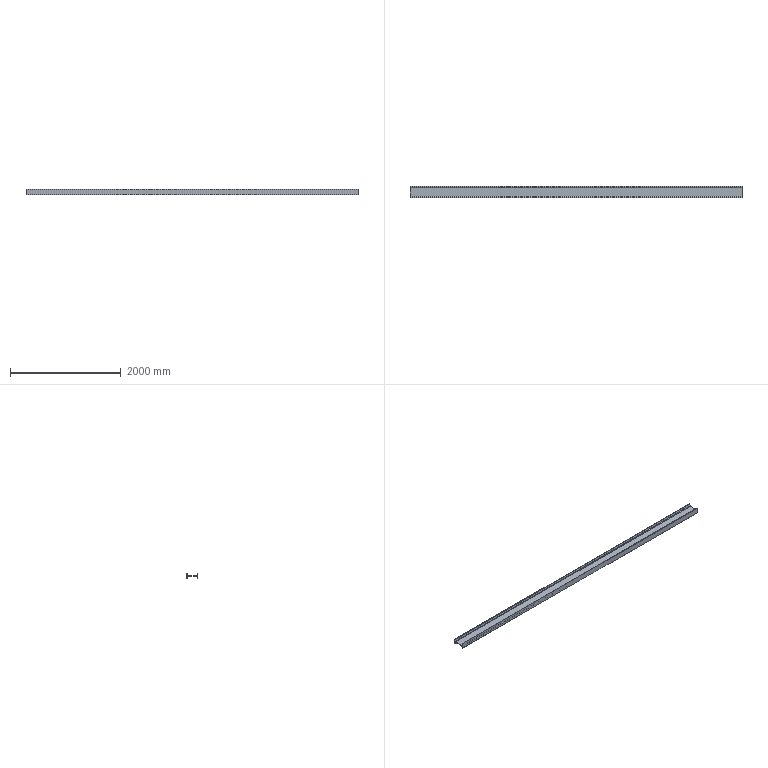Part | STEP file | E3-导轨工字钢2_Default<As Machined> | 1 solid | 46 faces | box 6000 x 200 x 102 mm | volume 23700400 mm3 | cylinder 32 | plane 14 | commonest cylinder face diameters 18 x28 9 x4